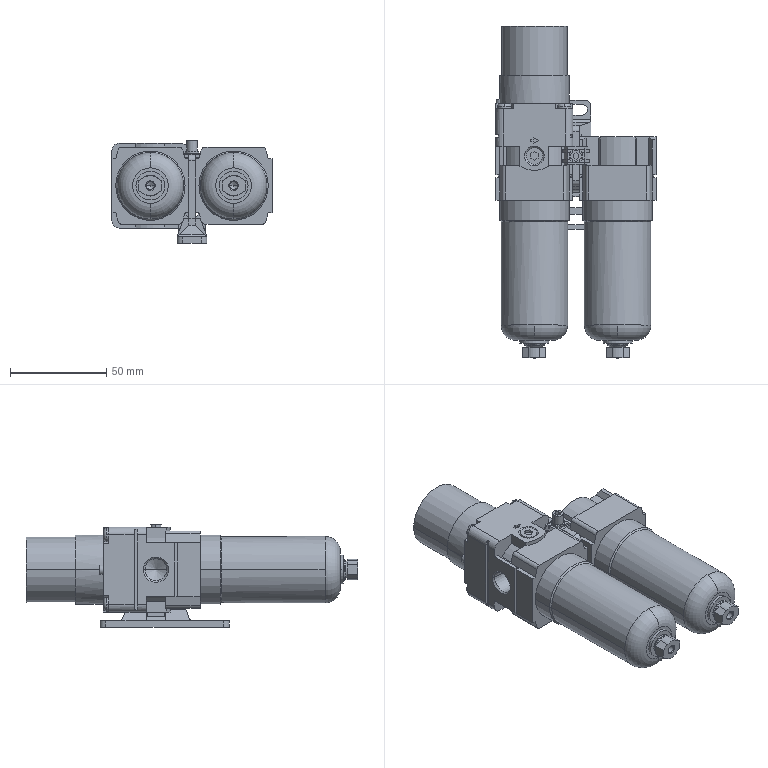Part | STEP file | AC20D-02C-A_0_^气源二联件-SMC | 9 solids | 485 faces | box 83.2 x 172.3 x 53.4 mm | volume 301660 mm3 | plane 302 | cylinder 111 | cone 52 | torus 20 | commonest cylinder face diameters 4 x10 7 x10 36 x10 3.242 x8 5.5 x8 11.445 x8